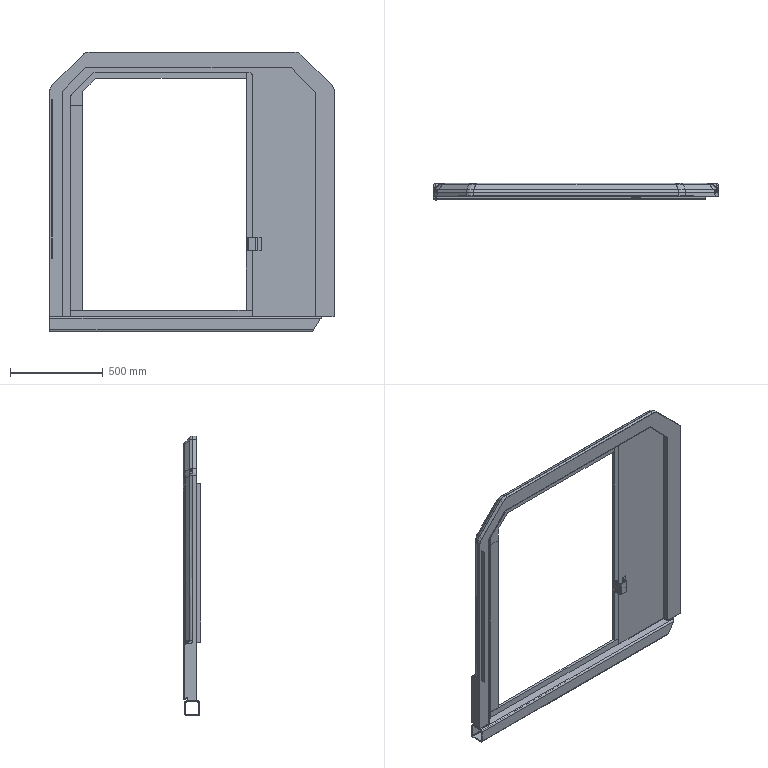Part | NX | features BREP 10 | 14 solids | 491 faces | box 1528 x 92.834 x 1503 mm | volume 10123824 mm3 | plane 251 | spline 132 | cylinder 84 | cone 24 | commonest cylinder face diameters 8 x16 9 x16 10 x15 20 x15 6 x8 13 x8